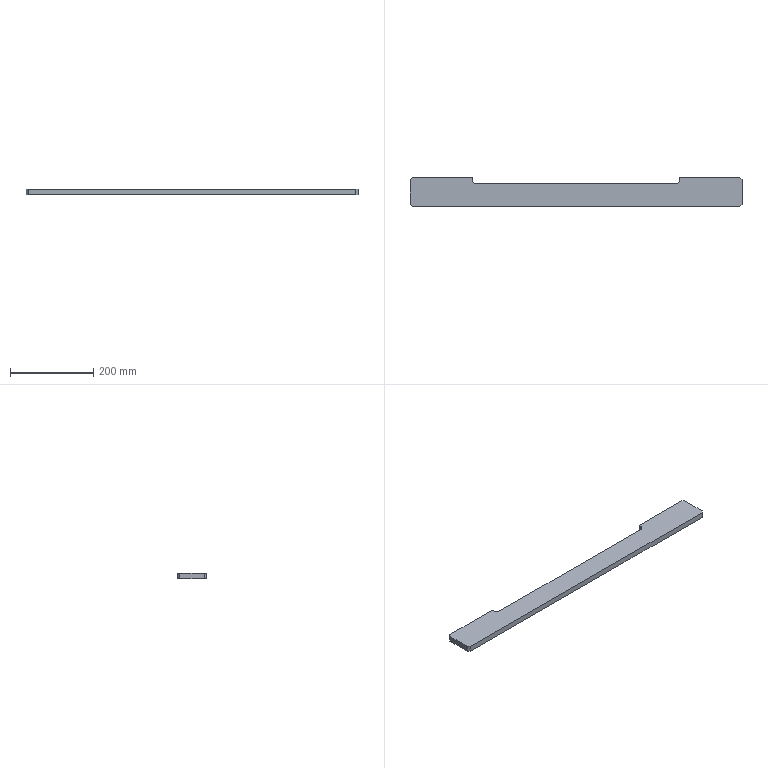Part | STEP file | 2012-06-08-01 | 1 solid | 16 faces | box 800 x 70 x 14 mm | volume 678901 mm3 | plane 14 | cylinder 2 | commonest cylinder face diameters 20 x2
STEP:
#1=CARTESIAN_POINT('',(0.,0.,0.));
#2=DIRECTION('',(0.,0.,1.));
#3=DIRECTION('',(1.,0.,0.));
#4=AXIS2_PLACEMENT_3D('',#1,#2,#3);
#5=CARTESIAN_POINT('',(-250.,35.,14.));
#6=VERTEX_POINT('',#5);
#7=CARTESIAN_POINT('',(-395.,35.,14.));
#8=VERTEX_POINT('',#7);
#9=CARTESIAN_POINT('',(-400.,35.,14.));
#10=DIRECTION('',(-1.,0.,0.));
#11=VECTOR('',#10,1.);
#12=LINE('',#9,#11);
#13=CARTESIAN_POINT('',(-400.,35.,14.));
#14=DIRECTION('',(0.,-1.,0.));
#15=DIRECTION('',(0.,0.,-1.));
#16=AXIS2_PLACEMENT_3D('',#13,#14,#15);
#17=PLANE('',#16);
#18=CARTESIAN_POINT('',(0.,0.));
#19=DIRECTION('',(0.,-1.));
#20=VECTOR('',#19,1.);
#21=LINE('',#18,#20);
#22=(GEOMETRIC_REPRESENTATION_CONTEXT(2)PARAMETRIC_REPRESENTATION_CONTEXT()REPRESENTATION_CONTEXT('',''));
#23=DEFINITIONAL_REPRESENTATION('',(#21),#22);
#24=PCURVE('',#17,#23);
#25=CARTESIAN_POINT('',(400.,-35.,14.));
#26=DIRECTION('',(0.,0.,1.));
#27=DIRECTION('',(1.,0.,0.));
#28=AXIS2_PLACEMENT_3D('',#25,#26,#27);
#29=PLANE('',#28);
#30=CARTESIAN_POINT('',(-800.,70.));
#31=DIRECTION('',(-1.,0.));
#32=VECTOR('',#31,1.);
#33=LINE('',#30,#32);
#34=(GEOMETRIC_REPRESENTATION_CONTEXT(2)PARAMETRIC_REPRESENTATION_CONTEXT()REPRESENTATION_CONTEXT('',''));
#35=DEFINITIONAL_REPRESENTATION('',(#33),#34);
#36=PCURVE('',#29,#35);
#37=SURFACE_CURVE('',#12,(#24,#36),.PCURVE_S1.);
#38=EDGE_CURVE('',#6,#8,#37,.T.);
#39=ORIENTED_EDGE('',*,*,#38,.F.);
#40=CARTESIAN_POINT('',(-250.,35.,0.));
#41=VERTEX_POINT('',#40);
#42=CARTESIAN_POINT('',(-250.,35.,-1.));
#43=DIRECTION('',(0.,0.,1.));
#44=VECTOR('',#43,1.);
#45=LINE('',#42,#44);
#46=CARTESIAN_POINT('',(15.,150.));
#47=DIRECTION('',(-1.,0.));
#48=VECTOR('',#47,1.);
#49=LINE('',#46,#48);
#50=(GEOMETRIC_REPRESENTATION_CONTEXT(2)PARAMETRIC_REPRESENTATION_CONTEXT()REPRESENTATION_CONTEXT('',''));
#51=DEFINITIONAL_REPRESENTATION('',(#49),#50);
#52=PCURVE('',#17,#51);
#53=CARTESIAN_POINT('',(-250.,35.,-1.));
#54=DIRECTION('',(-1.,0.,0.));
#55=DIRECTION('',(0.,0.,1.));
#56=AXIS2_PLACEMENT_3D('',#53,#54,#55);
#57=PLANE('',#56);
#58=CARTESIAN_POINT('',(0.,0.));
#59=DIRECTION('',(1.,0.));
#60=VECTOR('',#59,1.);
#61=LINE('',#58,#60);
#62=(GEOMETRIC_REPRESENTATION_CONTEXT(2)PARAMETRIC_REPRESENTATION_CONTEXT()REPRESENTATION_CONTEXT('',''));
#63=DEFINITIONAL_REPRESENTATION('',(#61),#62);
#64=PCURVE('',#57,#63);
#65=SURFACE_CURVE('',#45,(#52,#64),.PCURVE_S1.);
#66=EDGE_CURVE('',#41,#6,#65,.T.);
#67=ORIENTED_EDGE('',*,*,#66,.F.);
#68=CARTESIAN_POINT('',(-395.,35.,0.));
#69=VERTEX_POINT('',#68);
#70=CARTESIAN_POINT('',(-400.,35.,0.));
#71=DIRECTION('',(-1.,0.,0.));
#72=VECTOR('',#71,1.);
#73=LINE('',#70,#72);
#74=CARTESIAN_POINT('',(14.,0.));
#75=DIRECTION('',(0.,-1.));
#76=VECTOR('',#75,1.);
#77=LINE('',#74,#76);
#78=(GEOMETRIC_REPRESENTATION_CONTEXT(2)PARAMETRIC_REPRESENTATION_CONTEXT()REPRESENTATION_CONTEXT('',''));
#79=DEFINITIONAL_REPRESENTATION('',(#77),#78);
#80=PCURVE('',#17,#79);
#81=CARTESIAN_POINT('',(400.,-35.,0.));
#82=DIRECTION('',(0.,0.,1.));
#83=DIRECTION('',(1.,0.,0.));
#84=AXIS2_PLACEMENT_3D('',#81,#82,#83);
#85=PLANE('',#84);
#86=CARTESIAN_POINT('',(-800.,70.));
#87=DIRECTION('',(-1.,0.));
#88=VECTOR('',#87,1.);
#89=LINE('',#86,#88);
#90=(GEOMETRIC_REPRESENTATION_CONTEXT(2)PARAMETRIC_REPRESENTATION_CONTEXT()REPRESENTATION_CONTEXT('',''));
#91=DEFINITIONAL_REPRESENTATION('',(#89),#90);
#92=PCURVE('',#85,#91);
#93=SURFACE_CURVE('',#73,(#80,#92),.PCURVE_S1.);
#94=EDGE_CURVE('',#41,#69,#93,.T.);
#95=ORIENTED_EDGE('',*,*,#94,.T.);
#96=CARTESIAN_POINT('',(-395.,35.,14.));
#97=DIRECTION('',(0.,0.,1.));
#98=VECTOR('',#97,1.);
#99=LINE('',#96,#98);
#100=CARTESIAN_POINT('',(0.,5.));
#101=DIRECTION('',(-1.,0.));
#102=VECTOR('',#101,1.);
#103=LINE('',#100,#102);
#104=(GEOMETRIC_REPRESENTATION_CONTEXT(2)PARAMETRIC_REPRESENTATION_CONTEXT()REPRESENTATION_CONTEXT('',''));
#105=DEFINITIONAL_REPRESENTATION('',(#103),#104);
#106=PCURVE('',#17,#105);
#107=CARTESIAN_POINT('',(-400.,30.,14.));
#108=DIRECTION('',(0.7071,-0.7071,0.));
#109=DIRECTION('',(0.7071,0.7071,0.));
#110=AXIS2_PLACEMENT_3D('',#107,#108,#109);
#111=PLANE('',#110);
#112=CARTESIAN_POINT('',(7.071,0.));
#113=DIRECTION('',(0.,1.));
#114=VECTOR('',#113,1.);
#115=LINE('',#112,#114);
#116=(GEOMETRIC_REPRESENTATION_CONTEXT(2)PARAMETRIC_REPRESENTATION_CONTEXT()REPRESENTATION_CONTEXT('',''));
#117=DEFINITIONAL_REPRESENTATION('',(#115),#116);
#118=PCURVE('',#111,#117);
#119=SURFACE_CURVE('',#99,(#106,#118),.PCURVE_S1.);
#120=EDGE_CURVE('',#69,#8,#119,.T.);
#121=ORIENTED_EDGE('',*,*,#120,.T.);
#122=EDGE_LOOP('',(#39,#67,#95,#121));
#123=FACE_BOUND('',#122,.T.);
#124=ADVANCED_FACE('',(#123),#17,.F.);
#125=CARTESIAN_POINT('',(400.,-30.,14.));
#126=VERTEX_POINT('',#125);
#127=CARTESIAN_POINT('',(400.,30.,14.));
#128=VERTEX_POINT('',#127);
#129=CARTESIAN_POINT('',(400.,35.,14.));
#130=DIRECTION('',(0.,1.,0.));
#131=VECTOR('',#130,1.);
#132=LINE('',#129,#131);
#133=CARTESIAN_POINT('',(400.,35.,14.));
#134=DIRECTION('',(-1.,0.,0.));
#135=DIRECTION('',(0.,0.,1.));
#136=AXIS2_PLACEMENT_3D('',#133,#134,#135);
#137=PLANE('',#136);
#138=CARTESIAN_POINT('',(0.,0.));
#139=DIRECTION('',(0.,1.));
#140=VECTOR('',#139,1.);
#141=LINE('',#138,#140);
#142=(GEOMETRIC_REPRESENTATION_CONTEXT(2)PARAMETRIC_REPRESENTATION_CONTEXT()REPRESENTATION_CONTEXT('',''));
#143=DEFINITIONAL_REPRESENTATION('',(#141),#142);
#144=PCURVE('',#137,#143);
#145=CARTESIAN_POINT('',(0.,70.));
#146=DIRECTION('',(0.,1.));
#147=VECTOR('',#146,1.);
#148=LINE('',#145,#147);
#149=(GEOMETRIC_REPRESENTATION_CONTEXT(2)PARAMETRIC_REPRESENTATION_CONTEXT()REPRESENTATION_CONTEXT('',''));
#150=DEFINITIONAL_REPRESENTATION('',(#148),#149);
#151=PCURVE('',#29,#150);
#152=SURFACE_CURVE('',#132,(#144,#151),.PCURVE_S1.);
#153=EDGE_CURVE('',#126,#128,#152,.T.);
#154=ORIENTED_EDGE('',*,*,#153,.F.);
#155=CARTESIAN_POINT('',(400.,-30.,0.));
#156=VERTEX_POINT('',#155);
#157=CARTESIAN_POINT('',(400.,-30.,14.));
#158=DIRECTION('',(0.,0.,-1.));
#159=VECTOR('',#158,1.);
#160=LINE('',#157,#159);
#161=CARTESIAN_POINT('',(0.,-65.));
#162=DIRECTION('',(-1.,0.));
#163=VECTOR('',#162,1.);
#164=LINE('',#161,#163);
#165=(GEOMETRIC_REPRESENTATION_CONTEXT(2)PARAMETRIC_REPRESENTATION_CONTEXT()REPRESENTATION_CONTEXT('',''));
#166=DEFINITIONAL_REPRESENTATION('',(#164),#165);
#167=PCURVE('',#137,#166);
#168=CARTESIAN_POINT('',(400.,-30.,14.));
#169=DIRECTION('',(-0.7071,0.7071,0.));
#170=DIRECTION('',(-0.7071,-0.7071,0.));
#171=AXIS2_PLACEMENT_3D('',#168,#169,#170);
#172=PLANE('',#171);
#173=CARTESIAN_POINT('',(0.,0.));
#174=DIRECTION('',(0.,-1.));
#175=VECTOR('',#174,1.);
#176=LINE('',#173,#175);
#177=(GEOMETRIC_REPRESENTATION_CONTEXT(2)PARAMETRIC_REPRESENTATION_CONTEXT()REPRESENTATION_CONTEXT('',''));
#178=DEFINITIONAL_REPRESENTATION('',(#176),#177);
#179=PCURVE('',#172,#178);
#180=SURFACE_CURVE('',#160,(#167,#179),.PCURVE_S1.);
#181=EDGE_CURVE('',#126,#156,#180,.T.);
#182=ORIENTED_EDGE('',*,*,#181,.T.);
#183=CARTESIAN_POINT('',(400.,30.,0.));
#184=VERTEX_POINT('',#183);
#185=CARTESIAN_POINT('',(400.,35.,0.));
#186=DIRECTION('',(0.,1.,0.));
#187=VECTOR('',#186,1.);
#188=LINE('',#185,#187);
#189=CARTESIAN_POINT('',(-14.,0.));
#190=DIRECTION('',(0.,1.));
#191=VECTOR('',#190,1.);
#192=LINE('',#189,#191);
#193=(GEOMETRIC_REPRESENTATION_CONTEXT(2)PARAMETRIC_REPRESENTATION_CONTEXT()REPRESENTATION_CONTEXT('',''));
#194=DEFINITIONAL_REPRESENTATION('',(#192),#193);
#195=PCURVE('',#137,#194);
#196=CARTESIAN_POINT('',(0.,70.));
#197=DIRECTION('',(0.,1.));
#198=VECTOR('',#197,1.);
#199=LINE('',#196,#198);
#200=(GEOMETRIC_REPRESENTATION_CONTEXT(2)PARAMETRIC_REPRESENTATION_CONTEXT()REPRESENTATION_CONTEXT('',''));
#201=DEFINITIONAL_REPRESENTATION('',(#199),#200);
#202=PCURVE('',#85,#201);
#203=SURFACE_CURVE('',#188,(#195,#202),.PCURVE_S1.);
#204=EDGE_CURVE('',#156,#184,#203,.T.);
#205=ORIENTED_EDGE('',*,*,#204,.T.);
#206=CARTESIAN_POINT('',(400.,30.,14.));
#207=DIRECTION('',(0.,0.,1.));
#208=VECTOR('',#207,1.);
#209=LINE('',#206,#208);
#210=CARTESIAN_POINT('',(0.,-5.));
#211=DIRECTION('',(1.,0.));
#212=VECTOR('',#211,1.);
#213=LINE('',#210,#212);
#214=(GEOMETRIC_REPRESENTATION_CONTEXT(2)PARAMETRIC_REPRESENTATION_CONTEXT()REPRESENTATION_CONTEXT('',''));
#215=DEFINITIONAL_REPRESENTATION('',(#213),#214);
#216=PCURVE('',#137,#215);
#217=CARTESIAN_POINT('',(395.,35.,14.));
#218=DIRECTION('',(-0.7071,-0.7071,0.));
#219=DIRECTION('',(0.7071,-0.7071,0.));
#220=AXIS2_PLACEMENT_3D('',#217,#218,#219);
#221=PLANE('',#220);
#222=CARTESIAN_POINT('',(7.071,0.));
#223=DIRECTION('',(0.,1.));
#224=VECTOR('',#223,1.);
#225=LINE('',#222,#224);
#226=(GEOMETRIC_REPRESENTATION_CONTEXT(2)PARAMETRIC_REPRESENTATION_CONTEXT()REPRESENTATION_CONTEXT('',''));
#227=DEFINITIONAL_REPRESENTATION('',(#225),#226);
#228=PCURVE('',#221,#227);
#229=SURFACE_CURVE('',#209,(#216,#228),.PCURVE_S1.);
#230=EDGE_CURVE('',#184,#128,#229,.T.);
#231=ORIENTED_EDGE('',*,*,#230,.T.);
#232=EDGE_LOOP('',(#154,#182,#205,#231));
#233=FACE_BOUND('',#232,.T.);
#234=ADVANCED_FACE('',(#233),#137,.F.);
#235=CARTESIAN_POINT('',(395.,35.,0.));
#236=VERTEX_POINT('',#235);
#237=CARTESIAN_POINT('',(250.,35.,0.));
#238=VERTEX_POINT('',#237);
#239=CARTESIAN_POINT('',(-400.,35.,0.));
#240=DIRECTION('',(-1.,0.,0.));
#241=VECTOR('',#240,1.);
#242=LINE('',#239,#241);
#243=CARTESIAN_POINT('',(-400.,35.,14.));
#244=DIRECTION('',(0.,-1.,0.));
#245=DIRECTION('',(0.,0.,-1.));
#246=AXIS2_PLACEMENT_3D('',#243,#244,#245);
#247=PLANE('',#246);
#248=CARTESIAN_POINT('',(14.,0.));
#249=DIRECTION('',(0.,-1.));
#250=VECTOR('',#249,1.);
#251=LINE('',#248,#250);
#252=(GEOMETRIC_REPRESENTATION_CONTEXT(2)PARAMETRIC_REPRESENTATION_CONTEXT()REPRESENTATION_CONTEXT('',''));
#253=DEFINITIONAL_REPRESENTATION('',(#251),#252);
#254=PCURVE('',#247,#253);
#255=CARTESIAN_POINT('',(-800.,70.));
#256=DIRECTION('',(-1.,0.));
#257=VECTOR('',#256,1.);
#258=LINE('',#255,#257);
#259=(GEOMETRIC_REPRESENTATION_CONTEXT(2)PARAMETRIC_REPRESENTATION_CONTEXT()REPRESENTATION_CONTEXT('',''));
#260=DEFINITIONAL_REPRESENTATION('',(#258),#259);
#261=PCURVE('',#85,#260);
#262=SURFACE_CURVE('',#242,(#254,#261),.PCURVE_S1.);
#263=EDGE_CURVE('',#236,#238,#262,.T.);
#264=ORIENTED_EDGE('',*,*,#263,.T.);
#265=CARTESIAN_POINT('',(250.,35.,14.));
#266=VERTEX_POINT('',#265);
#267=CARTESIAN_POINT('',(250.,35.,-1.));
#268=DIRECTION('',(0.,0.,1.));
#269=VECTOR('',#268,1.);
#270=LINE('',#267,#269);
#271=CARTESIAN_POINT('',(15.,650.));
#272=DIRECTION('',(-1.,0.));
#273=VECTOR('',#272,1.);
#274=LINE('',#271,#273);
#275=(GEOMETRIC_REPRESENTATION_CONTEXT(2)PARAMETRIC_REPRESENTATION_CONTEXT()REPRESENTATION_CONTEXT('',''));
#276=DEFINITIONAL_REPRESENTATION('',(#274),#275);
#277=PCURVE('',#247,#276);
#278=CARTESIAN_POINT('',(250.,35.,-1.));
#279=DIRECTION('',(1.,0.,0.));
#280=DIRECTION('',(0.,0.,-1.));
#281=AXIS2_PLACEMENT_3D('',#278,#279,#280);
#282=PLANE('',#281);
#283=CARTESIAN_POINT('',(0.,0.));
#284=DIRECTION('',(-1.,0.));
#285=VECTOR('',#284,1.);
#286=LINE('',#283,#285);
#287=(GEOMETRIC_REPRESENTATION_CONTEXT(2)PARAMETRIC_REPRESENTATION_CONTEXT()REPRESENTATION_CONTEXT('',''));
#288=DEFINITIONAL_REPRESENTATION('',(#286),#287);
#289=PCURVE('',#282,#288);
#290=SURFACE_CURVE('',#270,(#277,#289),.PCURVE_S1.);
#291=EDGE_CURVE('',#238,#266,#290,.T.);
#292=ORIENTED_EDGE('',*,*,#291,.T.);
#293=CARTESIAN_POINT('',(395.,35.,14.));
#294=VERTEX_POINT('',#293);
#295=CARTESIAN_POINT('',(-400.,35.,14.));
#296=DIRECTION('',(-1.,0.,0.));
#297=VECTOR('',#296,1.);
#298=LINE('',#295,#297);
#299=CARTESIAN_POINT('',(0.,0.));
#300=DIRECTION('',(0.,-1.));
#301=VECTOR('',#300,1.);
#302=LINE('',#299,#301);
#303=(GEOMETRIC_REPRESENTATION_CONTEXT(2)PARAMETRIC_REPRESENTATION_CONTEXT()REPRESENTATION_CONTEXT('',''));
#304=DEFINITIONAL_REPRESENTATION('',(#302),#303);
#305=PCURVE('',#247,#304);
#306=CARTESIAN_POINT('',(-800.,70.));
#307=DIRECTION('',(-1.,0.));
#308=VECTOR('',#307,1.);
#309=LINE('',#306,#308);
#310=(GEOMETRIC_REPRESENTATION_CONTEXT(2)PARAMETRIC_REPRESENTATION_CONTEXT()REPRESENTATION_CONTEXT('',''));
#311=DEFINITIONAL_REPRESENTATION('',(#309),#310);
#312=PCURVE('',#29,#311);
#313=SURFACE_CURVE('',#298,(#305,#312),.PCURVE_S1.);
#314=EDGE_CURVE('',#294,#266,#313,.T.);
#315=ORIENTED_EDGE('',*,*,#314,.F.);
#316=CARTESIAN_POINT('',(395.,35.,14.));
#317=DIRECTION('',(0.,0.,-1.));
#318=VECTOR('',#317,1.);
#319=LINE('',#316,#318);
#320=CARTESIAN_POINT('',(0.,795.));
#321=DIRECTION('',(1.,0.));
#322=VECTOR('',#321,1.);
#323=LINE('',#320,#322);
#324=(GEOMETRIC_REPRESENTATION_CONTEXT(2)PARAMETRIC_REPRESENTATION_CONTEXT()REPRESENTATION_CONTEXT('',''));
#325=DEFINITIONAL_REPRESENTATION('',(#323),#324);
#326=PCURVE('',#247,#325);
#327=CARTESIAN_POINT('',(0.,0.));
#328=DIRECTION('',(0.,-1.));
#329=VECTOR('',#328,1.);
#330=LINE('',#327,#329);
#331=(GEOMETRIC_REPRESENTATION_CONTEXT(2)PARAMETRIC_REPRESENTATION_CONTEXT()REPRESENTATION_CONTEXT('',''));
#332=DEFINITIONAL_REPRESENTATION('',(#330),#331);
#333=PCURVE('',#221,#332);
#334=SURFACE_CURVE('',#319,(#326,#333),.PCURVE_S1.);
#335=EDGE_CURVE('',#294,#236,#334,.T.);
#336=ORIENTED_EDGE('',*,*,#335,.T.);
#337=EDGE_LOOP('',(#264,#292,#315,#336));
#338=FACE_BOUND('',#337,.T.);
#339=ADVANCED_FACE('',(#338),#247,.F.);
#340=CARTESIAN_POINT('',(-400.,30.,0.));
#341=VERTEX_POINT('',#340);
#342=CARTESIAN_POINT('',(-400.,-30.,0.));
#343=VERTEX_POINT('',#342);
#344=CARTESIAN_POINT('',(-400.,35.,0.));
#345=DIRECTION('',(0.,-1.,0.));
#346=VECTOR('',#345,1.);
#347=LINE('',#344,#346);
#348=CARTESIAN_POINT('',(-400.,35.,14.));
#349=DIRECTION('',(1.,0.,0.));
#350=DIRECTION('',(0.,0.,-1.));
#351=AXIS2_PLACEMENT_3D('',#348,#349,#350);
#352=PLANE('',#351);
#353=CARTESIAN_POINT('',(14.,0.));
#354=DIRECTION('',(0.,-1.));
#355=VECTOR('',#354,1.);
#356=LINE('',#353,#355);
#357=(GEOMETRIC_REPRESENTATION_CONTEXT(2)PARAMETRIC_REPRESENTATION_CONTEXT()REPRESENTATION_CONTEXT('',''));
#358=DEFINITIONAL_REPRESENTATION('',(#356),#357);
#359=PCURVE('',#352,#358);
#360=CARTESIAN_POINT('',(-800.,70.));
#361=DIRECTION('',(0.,-1.));
#362=VECTOR('',#361,1.);
#363=LINE('',#360,#362);
#364=(GEOMETRIC_REPRESENTATION_CONTEXT(2)PARAMETRIC_REPRESENTATION_CONTEXT()REPRESENTATION_CONTEXT('',''));
#365=DEFINITIONAL_REPRESENTATION('',(#363),#364);
#366=PCURVE('',#85,#365);
#367=SURFACE_CURVE('',#347,(#359,#366),.PCURVE_S1.);
#368=EDGE_CURVE('',#341,#343,#367,.T.);
#369=ORIENTED_EDGE('',*,*,#368,.T.);
#370=CARTESIAN_POINT('',(-400.,-30.,14.));
#371=VERTEX_POINT('',#370);
#372=CARTESIAN_POINT('',(-400.,-30.,14.));
#373=DIRECTION('',(0.,0.,1.));
#374=VECTOR('',#373,1.);
#375=LINE('',#372,#374);
#376=CARTESIAN_POINT('',(0.,-65.));
#377=DIRECTION('',(-1.,0.));
#378=VECTOR('',#377,1.);
#379=LINE('',#376,#378);
#380=(GEOMETRIC_REPRESENTATION_CONTEXT(2)PARAMETRIC_REPRESENTATION_CONTEXT()REPRESENTATION_CONTEXT('',''));
#381=DEFINITIONAL_REPRESENTATION('',(#379),#380);
#382=PCURVE('',#352,#381);
#383=CARTESIAN_POINT('',(-395.,-35.,14.));
#384=DIRECTION('',(0.7071,0.7071,0.));
#385=DIRECTION('',(-0.7071,0.7071,0.));
#386=AXIS2_PLACEMENT_3D('',#383,#384,#385);
#387=PLANE('',#386);
#388=CARTESIAN_POINT('',(7.071,0.));
#389=DIRECTION('',(0.,1.));
#390=VECTOR('',#389,1.);
#391=LINE('',#388,#390);
#392=(GEOMETRIC_REPRESENTATION_CONTEXT(2)PARAMETRIC_REPRESENTATION_CONTEXT()REPRESENTATION_CONTEXT('',''));
#393=DEFINITIONAL_REPRESENTATION('',(#391),#392);
#394=PCURVE('',#387,#393);
#395=SURFACE_CURVE('',#375,(#382,#394),.PCURVE_S1.);
#396=EDGE_CURVE('',#343,#371,#395,.T.);
#397=ORIENTED_EDGE('',*,*,#396,.T.);
#398=CARTESIAN_POINT('',(-400.,30.,14.));
#399=VERTEX_POINT('',#398);
#400=CARTESIAN_POINT('',(-400.,35.,14.));
#401=DIRECTION('',(0.,-1.,0.));
#402=VECTOR('',#401,1.);
#403=LINE('',#400,#402);
#404=CARTESIAN_POINT('',(0.,0.));
#405=DIRECTION('',(0.,-1.));
#406=VECTOR('',#405,1.);
#407=LINE('',#404,#406);
#408=(GEOMETRIC_REPRESENTATION_CONTEXT(2)PARAMETRIC_REPRESENTATION_CONTEXT()REPRESENTATION_CONTEXT('',''));
#409=DEFINITIONAL_REPRESENTATION('',(#407),#408);
#410=PCURVE('',#352,#409);
#411=CARTESIAN_POINT('',(-800.,70.));
#412=DIRECTION('',(0.,-1.));
#413=VECTOR('',#412,1.);
#414=LINE('',#411,#413);
#415=(GEOMETRIC_REPRESENTATION_CONTEXT(2)PARAMETRIC_REPRESENTATION_CONTEXT()REPRESENTATION_CONTEXT('',''));
#416=DEFINITIONAL_REPRESENTATION('',(#414),#415);
#417=PCURVE('',#29,#416);
#418=SURFACE_CURVE('',#403,(#410,#417),.PCURVE_S1.);
#419=EDGE_CURVE('',#399,#371,#418,.T.);
#420=ORIENTED_EDGE('',*,*,#419,.F.);
#421=CARTESIAN_POINT('',(-400.,30.,14.));
#422=DIRECTION('',(0.,0.,-1.));
#423=VECTOR('',#422,1.);
#424=LINE('',#421,#423);
#425=CARTESIAN_POINT('',(0.,-5.));
#426=DIRECTION('',(1.,0.));
#427=VECTOR('',#426,1.);
#428=LINE('',#425,#427);
#429=(GEOMETRIC_REPRESENTATION_CONTEXT(2)PARAMETRIC_REPRESENTATION_CONTEXT()REPRESENTATION_CONTEXT('',''));
#430=DEFINITIONAL_REPRESENTATION('',(#428),#429);
#431=PCURVE('',#352,#430);
#432=CARTESIAN_POINT('',(0.,0.));
#433=DIRECTION('',(0.,-1.));
#434=VECTOR('',#433,1.);
#435=LINE('',#432,#434);
#436=(GEOMETRIC_REPRESENTATION_CONTEXT(2)PARAMETRIC_REPRESENTATION_CONTEXT()REPRESENTATION_CONTEXT('',''));
#437=DEFINITIONAL_REPRESENTATION('',(#435),#436);
#438=PCURVE('',#111,#437);
#439=SURFACE_CURVE('',#424,(#431,#438),.PCURVE_S1.);
#440=EDGE_CURVE('',#399,#341,#439,.T.);
#441=ORIENTED_EDGE('',*,*,#440,.T.);
#442=EDGE_LOOP('',(#369,#397,#420,#441));
#443=FACE_BOUND('',#442,.T.);
#444=ADVANCED_FACE('',(#443),#352,.F.);
#445=CARTESIAN_POINT('',(-395.,-35.,14.));
#446=VERTEX_POINT('',#445);
#447=CARTESIAN_POINT('',(395.,-35.,14.));
#448=VERTEX_POINT('',#447);
#449=CARTESIAN_POINT('',(-400.,-35.,14.));
#450=DIRECTION('',(1.,0.,0.));
#451=VECTOR('',#450,1.);
#452=LINE('',#449,#451);
#453=CARTESIAN_POINT('',(-400.,-35.,14.));
#454=DIRECTION('',(0.,1.,0.));
#455=DIRECTION('',(0.,0.,1.));
#456=AXIS2_PLACEMENT_3D('',#453,#454,#455);
#457=PLANE('',#456);
#458=CARTESIAN_POINT('',(0.,0.));
#459=DIRECTION('',(0.,1.));
#460=VECTOR('',#459,1.);
#461=LINE('',#458,#460);
#462=(GEOMETRIC_REPRESENTATION_CONTEXT(2)PARAMETRIC_REPRESENTATION_CONTEXT()REPRESENTATION_CONTEXT('',''));
#463=DEFINITIONAL_REPRESENTATION('',(#461),#462);
#464=PCURVE('',#457,#463);
#465=CARTESIAN_POINT('',(-800.,0.));
#466=DIRECTION('',(1.,0.));
#467=VECTOR('',#466,1.);
#468=LINE('',#465,#467);
#469=(GEOMETRIC_REPRESENTATION_CONTEXT(2)PARAMETRIC_REPRESENTATION_CONTEXT()REPRESENTATION_CONTEXT('',''));
#470=DEFINITIONAL_REPRESENTATION('',(#468),#469);
#471=PCURVE('',#29,#470);
#472=SURFACE_CURVE('',#452,(#464,#471),.PCURVE_S1.);
#473=EDGE_CURVE('',#446,#448,#472,.T.);
#474=ORIENTED_EDGE('',*,*,#473,.F.);
#475=CARTESIAN_POINT('',(-395.,-35.,0.));
#476=VERTEX_POINT('',#475);
#477=CARTESIAN_POINT('',(-395.,-35.,14.));
#478=DIRECTION('',(0.,0.,-1.));
#479=VECTOR('',#478,1.);
#480=LINE('',#477,#479);
#481=CARTESIAN_POINT('',(0.,5.));
#482=DIRECTION('',(-1.,0.));
#483=VECTOR('',#482,1.);
#484=LINE('',#481,#483);
#485=(GEOMETRIC_REPRESENTATION_CONTEXT(2)PARAMETRIC_REPRESENTATION_CONTEXT()REPRESENTATION_CONTEXT('',''));
#486=DEFINITIONAL_REPRESENTATION('',(#484),#485);
#487=PCURVE('',#457,#486);
#488=CARTESIAN_POINT('',(0.,0.));
#489=DIRECTION('',(0.,-1.));
#490=VECTOR('',#489,1.);
#491=LINE('',#488,#490);
#492=(GEOMETRIC_REPRESENTATION_CONTEXT(2)PARAMETRIC_REPRESENTATION_CONTEXT()REPRESENTATION_CONTEXT('',''));
#493=DEFINITIONAL_REPRESENTATION('',(#491),#492);
#494=PCURVE('',#387,#493);
#495=SURFACE_CURVE('',#480,(#487,#494),.PCURVE_S1.);
#496=EDGE_CURVE('',#446,#476,#495,.T.);
#497=ORIENTED_EDGE('',*,*,#496,.T.);
#498=CARTESIAN_POINT('',(395.,-35.,0.));
#499=VERTEX_POINT('',#498);
#500=CARTESIAN_POINT('',(-400.,-35.,0.));
#501=DIRECTION('',(1.,0.,0.));
#502=VECTOR('',#501,1.);
#503=LINE('',#500,#502);
#504=CARTESIAN_POINT('',(-14.,0.));
#505=DIRECTION('',(0.,1.));
#506=VECTOR('',#505,1.);
#507=LINE('',#504,#506);
#508=(GEOMETRIC_REPRESENTATION_CONTEXT(2)PARAMETRIC_REPRESENTATION_CONTEXT()REPRESENTATION_CONTEXT('',''));
#509=DEFINITIONAL_REPRESENTATION('',(#507),#508);
#510=PCURVE('',#457,#509);
#511=CARTESIAN_POINT('',(-800.,0.));
#512=DIRECTION('',(1.,0.));
#513=VECTOR('',#512,1.);
#514=LINE('',#511,#513);
#515=(GEOMETRIC_REPRESENTATION_CONTEXT(2)PARAMETRIC_REPRESENTATION_CONTEXT()REPRESENTATION_CONTEXT('',''));
#516=DEFINITIONAL_REPRESENTATION('',(#514),#515);
#517=PCURVE('',#85,#516);
#518=SURFACE_CURVE('',#503,(#510,#517),.PCURVE_S1.);
#519=EDGE_CURVE('',#476,#499,#518,.T.);
#520=ORIENTED_EDGE('',*,*,#519,.T.);
#521=CARTESIAN_POINT('',(395.,-35.,14.));
#522=DIRECTION('',(0.,0.,1.));
#523=VECTOR('',#522,1.);
#524=LINE('',#521,#523);
#525=CARTESIAN_POINT('',(0.,795.));
#526=DIRECTION('',(1.,0.));
#527=VECTOR('',#526,1.);
#528=LINE('',#525,#527);
#529=(GEOMETRIC_REPRESENTATION_CONTEXT(2)PARAMETRIC_REPRESENTATION_CONTEXT()REPRESENTATION_CONTEXT('',''));
#530=DEFINITIONAL_REPRESENTATION('',(#528),#529);
#531=PCURVE('',#457,#530);
#532=CARTESIAN_POINT('',(7.071,0.));
#533=DIRECTION('',(0.,1.));
#534=VECTOR('',#533,1.);
#535=LINE('',#532,#534);
#536=(GEOMETRIC_REPRESENTATION_CONTEXT(2)PARAMETRIC_REPRESENTATION_CONTEXT()REPRESENTATION_CONTEXT('',''));
#537=DEFINITIONAL_REPRESENTATION('',(#535),#536);
#538=PCURVE('',#172,#537);
#539=SURFACE_CURVE('',#524,(#531,#538),.PCURVE_S1.);
#540=EDGE_CURVE('',#499,#448,#539,.T.);
#541=ORIENTED_EDGE('',*,*,#540,.T.);
#542=EDGE_LOOP('',(#474,#497,#520,#541));
#543=FACE_BOUND('',#542,.T.);
#544=ADVANCED_FACE('',(#543),#457,.F.);
#545=CARTESIAN_POINT('',(-250.,30.,14.));
#546=VERTEX_POINT('',#545);
#547=CARTESIAN_POINT('',(-250.,35.,14.));
#548=DIRECTION('',(0.,-1.,0.));
#549=VECTOR('',#548,1.);
#550=LINE('',#547,#549);
#551=CARTESIAN_POINT('',(-650.,70.));
#552=DIRECTION('',(0.,-1.));
#553=VECTOR('',#552,1.);
#554=LINE('',#551,#553);
#555=(GEOMETRIC_REPRESENTATION_CONTEXT(2)PARAMETRIC_REPRESENTATION_CONTEXT()REPRESENTATION_CONTEXT('',''));
#556=DEFINITIONAL_REPRESENTATION('',(#554),#555);
#557=PCURVE('',#29,#556);
#558=CARTESIAN_POINT('',(15.,0.));
#559=DIRECTION('',(0.,-1.));
#560=VECTOR('',#559,1.);
#561=LINE('',#558,#560);
#562=(GEOMETRIC_REPRESENTATION_CONTEXT(2)PARAMETRIC_REPRESENTATION_CONTEXT()REPRESENTATION_CONTEXT('',''));
#563=DEFINITIONAL_REPRESENTATION('',(#561),#562);
#564=PCURVE('',#57,#563);
#565=SURFACE_CURVE('',#550,(#557,#564),.PCURVE_S1.);
#566=EDGE_CURVE('',#6,#546,#565,.T.);
#567=ORIENTED_EDGE('',*,*,#566,.F.);
#568=ORIENTED_EDGE('',*,*,#38,.T.);
#569=CARTESIAN_POINT('',(-32.5,397.5,14.));
#570=DIRECTION('',(-0.7071,-0.7071,0.));
#571=VECTOR('',#570,1.);
#572=LINE('',#569,#571);
#573=CARTESIAN_POINT('',(-432.5,432.5));
#574=DIRECTION('',(-0.7071,-0.7071));
#575=VECTOR('',#574,1.);
#576=LINE('',#573,#575);
#577=(GEOMETRIC_REPRESENTATION_CONTEXT(2)PARAMETRIC_REPRESENTATION_CONTEXT()REPRESENTATION_CONTEXT('',''));
#578=DEFINITIONAL_REPRESENTATION('',(#576),#577);
#579=PCURVE('',#29,#578);
#580=CARTESIAN_POINT('',(519.723,0.));
#581=DIRECTION('',(-1.,0.));
#582=VECTOR('',#581,1.);
#583=LINE('',#580,#582);
#584=(GEOMETRIC_REPRESENTATION_CONTEXT(2)PARAMETRIC_REPRESENTATION_CONTEXT()REPRESENTATION_CONTEXT('',''));
#585=DEFINITIONAL_REPRESENTATION('',(#583),#584);
#586=PCURVE('',#111,#585);
#587=SURFACE_CURVE('',#572,(#579,#586),.PCURVE_S1.);
#588=EDGE_CURVE('',#8,#399,#587,.T.);
#589=ORIENTED_EDGE('',*,*,#588,.T.);
#590=ORIENTED_EDGE('',*,*,#419,.T.);
#591=CARTESIAN_POINT('',(2.5,-432.5,14.));
#592=DIRECTION('',(0.7071,-0.7071,0.));
#593=VECTOR('',#592,1.);
#594=LINE('',#591,#593);
#595=CARTESIAN_POINT('',(-397.5,-397.5));
#596=DIRECTION('',(0.7071,-0.7071));
#597=VECTOR('',#596,1.);
#598=LINE('',#595,#597);
#599=(GEOMETRIC_REPRESENTATION_CONTEXT(2)PARAMETRIC_REPRESENTATION_CONTEXT()REPRESENTATION_CONTEXT('',''));
#600=DEFINITIONAL_REPRESENTATION('',(#598),#599);
#601=PCURVE('',#29,#600);
#602=CARTESIAN_POINT('',(-562.15,0.));
#603=DIRECTION('',(-1.,0.));
#604=VECTOR('',#603,1.);
#605=LINE('',#602,#604);
#606=(GEOMETRIC_REPRESENTATION_CONTEXT(2)PARAMETRIC_REPRESENTATION_CONTEXT()REPRESENTATION_CONTEXT('',''));
#607=DEFINITIONAL_REPRESENTATION('',(#605),#606);
#608=PCURVE('',#387,#607);
#609=SURFACE_CURVE('',#594,(#601,#608),.PCURVE_S1.);
#610=EDGE_CURVE('',#371,#446,#609,.T.);
#611=ORIENTED_EDGE('',*,*,#610,.T.);
#612=ORIENTED_EDGE('',*,*,#473,.T.);
#613=CARTESIAN_POINT('',(397.5,-32.5,14.));
#614=DIRECTION('',(0.7071,0.7071,0.));
#615=VECTOR('',#614,1.);
#616=LINE('',#613,#615);
#617=CARTESIAN_POINT('',(-2.5,2.5));
#618=DIRECTION('',(0.7071,0.7071));
#619=VECTOR('',#618,1.);
#620=LINE('',#617,#619);
#621=(GEOMETRIC_REPRESENTATION_CONTEXT(2)PARAMETRIC_REPRESENTATION_CONTEXT()REPRESENTATION_CONTEXT('',''));
#622=DEFINITIONAL_REPRESENTATION('',(#620),#621);
#623=PCURVE('',#29,#622);
#624=CARTESIAN_POINT('',(3.536,0.));
#625=DIRECTION('',(-1.,0.));
#626=VECTOR('',#625,1.);
#627=LINE('',#624,#626);
#628=(GEOMETRIC_REPRESENTATION_CONTEXT(2)PARAMETRIC_REPRESENTATION_CONTEXT()REPRESENTATION_CONTEXT('',''));
#629=DEFINITIONAL_REPRESENTATION('',(#627),#628);
#630=PCURVE('',#172,#629);
#631=SURFACE_CURVE('',#616,(#623,#630),.PCURVE_S1.);
#632=EDGE_CURVE('',#448,#126,#631,.T.);
#633=ORIENTED_EDGE('',*,*,#632,.T.);
#634=ORIENTED_EDGE('',*,*,#153,.T.);
#635=CARTESIAN_POINT('',(432.5,-2.5,14.));
#636=DIRECTION('',(-0.7071,0.7071,0.));
#637=VECTOR('',#636,1.);
#638=LINE('',#635,#637);
#639=CARTESIAN_POINT('',(32.5,32.5));
#640=DIRECTION('',(-0.7071,0.7071));
#641=VECTOR('',#640,1.);
#642=LINE('',#639,#641);
#643=(GEOMETRIC_REPRESENTATION_CONTEXT(2)PARAMETRIC_REPRESENTATION_CONTEXT()REPRESENTATION_CONTEXT('',''));
#644=DEFINITIONAL_REPRESENTATION('',(#642),#643);
#645=PCURVE('',#29,#644);
#646=CARTESIAN_POINT('',(53.033,0.));
#647=DIRECTION('',(-1.,0.));
#648=VECTOR('',#647,1.);
#649=LINE('',#646,#648);
#650=(GEOMETRIC_REPRESENTATION_CONTEXT(2)PARAMETRIC_REPRESENTATION_CONTEXT()REPRESENTATION_CONTEXT('',''));
#651=DEFINITIONAL_REPRESENTATION('',(#649),#650);
#652=PCURVE('',#221,#651);
#653=SURFACE_CURVE('',#638,(#645,#652),.PCURVE_S1.);
#654=EDGE_CURVE('',#128,#294,#653,.T.);
#655=ORIENTED_EDGE('',*,*,#654,.T.);
#656=ORIENTED_EDGE('',*,*,#314,.T.);
#657=CARTESIAN_POINT('',(250.,30.,14.));
#658=VERTEX_POINT('',#657);
#659=CARTESIAN_POINT('',(250.,35.,14.));
#660=DIRECTION('',(0.,1.,0.));
#661=VECTOR('',#660,1.);
#662=LINE('',#659,#661);
#663=CARTESIAN_POINT('',(-150.,70.));
#664=DIRECTION('',(0.,1.));
#665=VECTOR('',#664,1.);
#666=LINE('',#663,#665);
#667=(GEOMETRIC_REPRESENTATION_CONTEXT(2)PARAMETRIC_REPRESENTATION_CONTEXT()REPRESENTATION_CONTEXT('',''));
#668=DEFINITIONAL_REPRESENTATION('',(#666),#667);
#669=PCURVE('',#29,#668);
#670=CARTESIAN_POINT('',(-15.,0.));
#671=DIRECTION('',(0.,1.));
#672=VECTOR('',#671,1.);
#673=LINE('',#670,#672);
#674=(GEOMETRIC_REPRESENTATION_CONTEXT(2)PARAMETRIC_REPRESENTATION_CONTEXT()REPRESENTATION_CONTEXT('',''));
#675=DEFINITIONAL_REPRESENTATION('',(#673),#674);
#676=PCURVE('',#282,#675);
#677=SURFACE_CURVE('',#662,(#669,#676),.PCURVE_S1.);
#678=EDGE_CURVE('',#658,#266,#677,.T.);
#679=ORIENTED_EDGE('',*,*,#678,.F.);
#680=CARTESIAN_POINT('',(240.,20.,14.));
#681=VERTEX_POINT('',#680);
#682=CARTESIAN_POINT('',(240.,30.,14.));
#683=DIRECTION('',(0.,0.,-1.));
#684=DIRECTION('',(1.,0.,0.));
#685=AXIS2_PLACEMENT_3D('',#682,#683,#684);
#686=CIRCLE('',#685,10.);
#687=CARTESIAN_POINT('',(-150.,65.));
#688=CARTESIAN_POINT('',(-150.,47.679));
#689=CARTESIAN_POINT('',(-165.,56.34));
#690=CARTESIAN_POINT('',(-180.,65.));
#691=CARTESIAN_POINT('',(-165.,73.66));
#692=CARTESIAN_POINT('',(-150.,82.321));
#693=CARTESIAN_POINT('',(-150.,65.));
#694=(BOUNDED_CURVE()B_SPLINE_CURVE(2,(#687,#688,#689,#690,#691,#692,#693),.UNSPECIFIED.,.T.,.F.)B_SPLINE_CURVE_WITH_KNOTS((1,2,2,2,2,1),(-2.094,0.,2.094,4.189,6.283,8.378),.UNSPECIFIED.)CURVE()GEOMETRIC_REPRESENTATION_ITEM()RATIONAL_B_SPLINE_CURVE((1.,0.5,1.,0.5,1.,0.5,1.))REPRESENTATION_ITEM(''));
#695=(GEOMETRIC_REPRESENTATION_CONTEXT(2)PARAMETRIC_REPRESENTATION_CONTEXT()REPRESENTATION_CONTEXT('',''));
#696=DEFINITIONAL_REPRESENTATION('',(#694),#695);
#697=PCURVE('',#29,#696);
#698=CARTESIAN_POINT('',(240.,30.,-1.));
#699=DIRECTION('',(0.,0.,-1.));
#700=DIRECTION('',(-1.,0.,0.));
#701=AXIS2_PLACEMENT_3D('',#698,#699,#700);
#702=CYLINDRICAL_SURFACE('',#701,10.);
#703=CARTESIAN_POINT('',(3.142,-15.));
#704=DIRECTION('',(1.,0.));
#705=VECTOR('',#704,1.);
#706=LINE('',#703,#705);
#707=(GEOMETRIC_REPRESENTATION_CONTEXT(2)PARAMETRIC_REPRESENTATION_CONTEXT()REPRESENTATION_CONTEXT('',''));
#708=DEFINITIONAL_REPRESENTATION('',(#706),#707);
#709=PCURVE('',#702,#708);
#710=SURFACE_CURVE('',#686,(#697,#709),.PCURVE_S1.);
#711=EDGE_CURVE('',#658,#681,#710,.T.);
#712=ORIENTED_EDGE('',*,*,#711,.T.);
#713=CARTESIAN_POINT('',(-240.,20.,14.));
#714=VERTEX_POINT('',#713);
#715=CARTESIAN_POINT('',(-250.,20.,14.));
#716=DIRECTION('',(1.,0.,0.));
#717=VECTOR('',#716,1.);
#718=LINE('',#715,#717);
#719=CARTESIAN_POINT('',(-650.,55.));
#720=DIRECTION('',(1.,0.));
#721=VECTOR('',#720,1.);
#722=LINE('',#719,#721);
#723=(GEOMETRIC_REPRESENTATION_CONTEXT(2)PARAMETRIC_REPRESENTATION_CONTEXT()REPRESENTATION_CONTEXT('',''));
#724=DEFINITIONAL_REPRESENTATION('',(#722),#723);
#725=PCURVE('',#29,#724);
#726=CARTESIAN_POINT('',(-250.,20.,-1.));
#727=DIRECTION('',(0.,-1.,0.));
#728=DIRECTION('',(1.,0.,0.));
#729=AXIS2_PLACEMENT_3D('',#726,#727,#728);
#730=PLANE('',#729);
#731=CARTESIAN_POINT('',(0.,15.));
#732=DIRECTION('',(1.,0.));
#733=VECTOR('',#732,1.);
#734=LINE('',#731,#733);
#735=(GEOMETRIC_REPRESENTATION_CONTEXT(2)PARAMETRIC_REPRESENTATION_CONTEXT()REPRESENTATION_CONTEXT('',''));
#736=DEFINITIONAL_REPRESENTATION('',(#734),#735);
#737=PCURVE('',#730,#736);
#738=SURFACE_CURVE('',#718,(#725,#737),.PCURVE_S1.);
#739=EDGE_CURVE('',#714,#681,#738,.T.);
#740=ORIENTED_EDGE('',*,*,#739,.F.);
#741=CARTESIAN_POINT('',(-240.,30.,14.));
#742=DIRECTION('',(0.,0.,-1.));
#743=DIRECTION('',(1.,0.,0.));
#744=AXIS2_PLACEMENT_3D('',#741,#742,#743);
#745=CIRCLE('',#744,10.);
#746=CARTESIAN_POINT('',(-630.,65.));
#747=CARTESIAN_POINT('',(-630.,47.679));
#748=CARTESIAN_POINT('',(-645.,56.34));
#749=CARTESIAN_POINT('',(-660.,65.));
#750=CARTESIAN_POINT('',(-645.,73.66));
#751=CARTESIAN_POINT('',(-630.,82.321));
#752=CARTESIAN_POINT('',(-630.,65.));
#753=(BOUNDED_CURVE()B_SPLINE_CURVE(2,(#746,#747,#748,#749,#750,#751,#752),.UNSPECIFIED.,.T.,.F.)B_SPLINE_CURVE_WITH_KNOTS((1,2,2,2,2,1),(-2.094,0.,2.094,4.189,6.283,8.378),.UNSPECIFIED.)CURVE()GEOMETRIC_REPRESENTATION_ITEM()RATIONAL_B_SPLINE_CURVE((1.,0.5,1.,0.5,1.,0.5,1.))REPRESENTATION_ITEM(''));
#754=(GEOMETRIC_REPRESENTATION_CONTEXT(2)PARAMETRIC_REPRESENTATION_CONTEXT()REPRESENTATION_CONTEXT('',''));
#755=DEFINITIONAL_REPRESENTATION('',(#753),#754);
#756=PCURVE('',#29,#755);
#757=CARTESIAN_POINT('',(-240.,30.,-1.));
#758=DIRECTION('',(0.,0.,-1.));
#759=DIRECTION('',(-1.,0.,0.));
#760=AXIS2_PLACEMENT_3D('',#757,#758,#759);
#761=CYLINDRICAL_SURFACE('',#760,10.);
#762=CARTESIAN_POINT('',(3.142,-15.));
#763=DIRECTION('',(1.,0.));
#764=VECTOR('',#763,1.);
#765=LINE('',#762,#764);
#766=(GEOMETRIC_REPRESENTATION_CONTEXT(2)PARAMETRIC_REPRESENTATION_CONTEXT()REPRESENTATION_CONTEXT('',''));
#767=DEFINITIONAL_REPRESENTATION('',(#765),#766);
#768=PCURVE('',#761,#767);
#769=SURFACE_CURVE('',#745,(#756,#768),.PCURVE_S1.);
#770=EDGE_CURVE('',#714,#546,#769,.T.);
#771=ORIENTED_EDGE('',*,*,#770,.T.);
#772=EDGE_LOOP('',(#567,#568,#589,#590,#611,#612,#633,#634,#655,#656,#679,#712,#740,#771));
#773=FACE_BOUND('',#772,.T.);
#774=ADVANCED_FACE('',(#773),#29,.T.);
#775=ORIENTED_EDGE('',*,*,#94,.F.);
#776=CARTESIAN_POINT('',(-250.,30.,0.));
#777=VERTEX_POINT('',#776);
#778=CARTESIAN_POINT('',(-250.,-35.,0.));
#779=DIRECTION('',(0.,-1.,0.));
#780=VECTOR('',#779,1.);
#781=LINE('',#778,#780);
#782=CARTESIAN_POINT('',(-650.,0.));
#783=DIRECTION('',(0.,-1.));
#784=VECTOR('',#783,1.);
#785=LINE('',#782,#784);
#786=(GEOMETRIC_REPRESENTATION_CONTEXT(2)PARAMETRIC_REPRESENTATION_CONTEXT()REPRESENTATION_CONTEXT('',''));
#787=DEFINITIONAL_REPRESENTATION('',(#785),#786);
#788=PCURVE('',#85,#787);
#789=CARTESIAN_POINT('',(1.,-70.));
#790=DIRECTION('',(0.,-1.));
#791=VECTOR('',#790,1.);
#792=LINE('',#789,#791);
#793=(GEOMETRIC_REPRESENTATION_CONTEXT(2)PARAMETRIC_REPRESENTATION_CONTEXT()REPRESENTATION_CONTEXT('',''));
#794=DEFINITIONAL_REPRESENTATION('',(#792),#793);
#795=PCURVE('',#57,#794);
#796=SURFACE_CURVE('',#781,(#788,#795),.PCURVE_S1.);
#797=EDGE_CURVE('',#41,#777,#796,.T.);
#798=ORIENTED_EDGE('',*,*,#797,.T.);
#799=CARTESIAN_POINT('',(-240.,20.,0.));
#800=VERTEX_POINT('',#799);
#801=CARTESIAN_POINT('',(-240.,30.,0.));
#802=DIRECTION('',(0.,0.,1.));
#803=DIRECTION('',(1.,0.,0.));
#804=AXIS2_PLACEMENT_3D('',#801,#802,#803);
#805=CIRCLE('',#804,10.);
#806=CARTESIAN_POINT('',(-640.,65.));
#807=DIRECTION('',(1.,0.));
#808=AXIS2_PLACEMENT_2D('',#806,#807);
#809=CIRCLE('',#808,10.);
#810=(GEOMETRIC_REPRESENTATION_CONTEXT(2)PARAMETRIC_REPRESENTATION_CONTEXT()REPRESENTATION_CONTEXT('',''));
#811=DEFINITIONAL_REPRESENTATION('',(#809),#810);
#812=PCURVE('',#85,#811);
#813=CARTESIAN_POINT('',(9.425,-1.));
#814=DIRECTION('',(-1.,0.));
#815=VECTOR('',#814,1.);
#816=LINE('',#813,#815);
#817=(GEOMETRIC_REPRESENTATION_CONTEXT(2)PARAMETRIC_REPRESENTATION_CONTEXT()REPRESENTATION_CONTEXT('',''));
#818=DEFINITIONAL_REPRESENTATION('',(#816),#817);
#819=PCURVE('',#761,#818);
#820=SURFACE_CURVE('',#805,(#812,#819),.PCURVE_S1.);
#821=EDGE_CURVE('',#777,#800,#820,.T.);
#822=ORIENTED_EDGE('',*,*,#821,.T.);
#823=CARTESIAN_POINT('',(240.,20.,0.));
#824=VERTEX_POINT('',#823);
#825=CARTESIAN_POINT('',(400.,20.,0.));
#826=DIRECTION('',(1.,0.,0.));
#827=VECTOR('',#826,1.);
#828=LINE('',#825,#827);
#829=CARTESIAN_POINT('',(0.,55.));
#830=DIRECTION('',(1.,0.));
#831=VECTOR('',#830,1.);
#832=LINE('',#829,#831);
#833=(GEOMETRIC_REPRESENTATION_CONTEXT(2)PARAMETRIC_REPRESENTATION_CONTEXT()REPRESENTATION_CONTEXT('',''));
#834=DEFINITIONAL_REPRESENTATION('',(#832),#833);
#835=PCURVE('',#85,#834);
#836=CARTESIAN_POINT('',(650.,1.));
#837=DIRECTION('',(1.,0.));
#838=VECTOR('',#837,1.);
#839=LINE('',#836,#838);
#840=(GEOMETRIC_REPRESENTATION_CONTEXT(2)PARAMETRIC_REPRESENTATION_CONTEXT()REPRESENTATION_CONTEXT('',''));
#841=DEFINITIONAL_REPRESENTATION('',(#839),#840);
#842=PCURVE('',#730,#841);
#843=SURFACE_CURVE('',#828,(#835,#842),.PCURVE_S1.);
#844=EDGE_CURVE('',#800,#824,#843,.T.);
#845=ORIENTED_EDGE('',*,*,#844,.T.);
#846=CARTESIAN_POINT('',(250.,30.,0.));
#847=VERTEX_POINT('',#846);
#848=CARTESIAN_POINT('',(240.,30.,0.));
#849=DIRECTION('',(0.,0.,1.));
#850=DIRECTION('',(1.,0.,0.));
#851=AXIS2_PLACEMENT_3D('',#848,#849,#850);
#852=CIRCLE('',#851,10.);
#853=CARTESIAN_POINT('',(-160.,65.));
#854=DIRECTION('',(1.,0.));
#855=AXIS2_PLACEMENT_2D('',#853,#854);
#856=CIRCLE('',#855,10.);
#857=(GEOMETRIC_REPRESENTATION_CONTEXT(2)PARAMETRIC_REPRESENTATION_CONTEXT()REPRESENTATION_CONTEXT('',''));
#858=DEFINITIONAL_REPRESENTATION('',(#856),#857);
#859=PCURVE('',#85,#858);
#860=CARTESIAN_POINT('',(9.425,-1.));
#861=DIRECTION('',(-1.,0.));
#862=VECTOR('',#861,1.);
#863=LINE('',#860,#862);
#864=(GEOMETRIC_REPRESENTATION_CONTEXT(2)PARAMETRIC_REPRESENTATION_CONTEXT()REPRESENTATION_CONTEXT('',''));
#865=DEFINITIONAL_REPRESENTATION('',(#863),#864);
#866=PCURVE('',#702,#865);
#867=SURFACE_CURVE('',#852,(#859,#866),.PCURVE_S1.);
#868=EDGE_CURVE('',#824,#847,#867,.T.);
#869=ORIENTED_EDGE('',*,*,#868,.T.);
#870=CARTESIAN_POINT('',(250.,-35.,0.));
#871=DIRECTION('',(0.,1.,0.));
#872=VECTOR('',#871,1.);
#873=LINE('',#870,#872);
#874=CARTESIAN_POINT('',(-150.,0.));
#875=DIRECTION('',(0.,1.));
#876=VECTOR('',#875,1.);
#877=LINE('',#874,#876);
#878=(GEOMETRIC_REPRESENTATION_CONTEXT(2)PARAMETRIC_REPRESENTATION_CONTEXT()REPRESENTATION_CONTEXT('',''));
#879=DEFINITIONAL_REPRESENTATION('',(#877),#878);
#880=PCURVE('',#85,#879);
#881=CARTESIAN_POINT('',(-1.,-70.));
#882=DIRECTION('',(0.,1.));
#883=VECTOR('',#882,1.);
#884=LINE('',#881,#883);
#885=(GEOMETRIC_REPRESENTATION_CONTEXT(2)PARAMETRIC_REPRESENTATION_CONTEXT()REPRESENTATION_CONTEXT('',''));
#886=DEFINITIONAL_REPRESENTATION('',(#884),#885);
#887=PCURVE('',#282,#886);
#888=SURFACE_CURVE('',#873,(#880,#887),.PCURVE_S1.);
#889=EDGE_CURVE('',#847,#238,#888,.T.);
#890=ORIENTED_EDGE('',*,*,#889,.T.);
#891=ORIENTED_EDGE('',*,*,#263,.F.);
#892=CARTESIAN_POINT('',(395.,35.,0.));
#893=DIRECTION('',(0.7071,-0.7071,0.));
#894=VECTOR('',#893,1.);
#895=LINE('',#892,#894);
#896=CARTESIAN_POINT('',(-5.,70.));
#897=DIRECTION('',(0.7071,-0.7071));
#898=VECTOR('',#897,1.);
#899=LINE('',#896,#898);
#900=(GEOMETRIC_REPRESENTATION_CONTEXT(2)PARAMETRIC_REPRESENTATION_CONTEXT()REPRESENTATION_CONTEXT('',''));
#901=DEFINITIONAL_REPRESENTATION('',(#899),#900);
#902=PCURVE('',#85,#901);
#903=CARTESIAN_POINT('',(0.,-14.));
#904=DIRECTION('',(1.,0.));
#905=VECTOR('',#904,1.);
#906=LINE('',#903,#905);
#907=(GEOMETRIC_REPRESENTATION_CONTEXT(2)PARAMETRIC_REPRESENTATION_CONTEXT()REPRESENTATION_CONTEXT('',''));
#908=DEFINITIONAL_REPRESENTATION('',(#906),#907);
#909=PCURVE('',#221,#908);
#910=SURFACE_CURVE('',#895,(#902,#909),.PCURVE_S1.);
#911=EDGE_CURVE('',#236,#184,#910,.T.);
#912=ORIENTED_EDGE('',*,*,#911,.T.);
#913=ORIENTED_EDGE('',*,*,#204,.F.);
#914=CARTESIAN_POINT('',(400.,-30.,0.));
#915=DIRECTION('',(-0.7071,-0.7071,0.));
#916=VECTOR('',#915,1.);
#917=LINE('',#914,#916);
#918=CARTESIAN_POINT('',(0.,5.));
#919=DIRECTION('',(-0.7071,-0.7071));
#920=VECTOR('',#919,1.);
#921=LINE('',#918,#920);
#922=(GEOMETRIC_REPRESENTATION_CONTEXT(2)PARAMETRIC_REPRESENTATION_CONTEXT()REPRESENTATION_CONTEXT('',''));
#923=DEFINITIONAL_REPRESENTATION('',(#921),#922);
#924=PCURVE('',#85,#923);
#925=CARTESIAN_POINT('',(0.,-14.));
#926=DIRECTION('',(1.,0.));
#927=VECTOR('',#926,1.);
#928=LINE('',#925,#927);
#929=(GEOMETRIC_REPRESENTATION_CONTEXT(2)PARAMETRIC_REPRESENTATION_CONTEXT()REPRESENTATION_CONTEXT('',''));
#930=DEFINITIONAL_REPRESENTATION('',(#928),#929);
#931=PCURVE('',#172,#930);
#932=SURFACE_CURVE('',#917,(#924,#931),.PCURVE_S1.);
#933=EDGE_CURVE('',#156,#499,#932,.T.);
#934=ORIENTED_EDGE('',*,*,#933,.T.);
#935=ORIENTED_EDGE('',*,*,#519,.F.);
#936=CARTESIAN_POINT('',(-395.,-35.,0.));
#937=DIRECTION('',(-0.7071,0.7071,0.));
#938=VECTOR('',#937,1.);
#939=LINE('',#936,#938);
#940=CARTESIAN_POINT('',(-795.,0.));
#941=DIRECTION('',(-0.7071,0.7071));
#942=VECTOR('',#941,1.);
#943=LINE('',#940,#942);
#944=(GEOMETRIC_REPRESENTATION_CONTEXT(2)PARAMETRIC_REPRESENTATION_CONTEXT()REPRESENTATION_CONTEXT('',''));
#945=DEFINITIONAL_REPRESENTATION('',(#943),#944);
#946=PCURVE('',#85,#945);
#947=CARTESIAN_POINT('',(0.,-14.));
#948=DIRECTION('',(1.,0.));
#949=VECTOR('',#948,1.);
#950=LINE('',#947,#949);
#951=(GEOMETRIC_REPRESENTATION_CONTEXT(2)PARAMETRIC_REPRESENTATION_CONTEXT()REPRESENTATION_CONTEXT('',''));
#952=DEFINITIONAL_REPRESENTATION('',(#950),#951);
#953=PCURVE('',#387,#952);
#954=SURFACE_CURVE('',#939,(#946,#953),.PCURVE_S1.);
#955=EDGE_CURVE('',#476,#343,#954,.T.);
#956=ORIENTED_EDGE('',*,*,#955,.T.);
#957=ORIENTED_EDGE('',*,*,#368,.F.);
#958=CARTESIAN_POINT('',(-400.,30.,0.));
#959=DIRECTION('',(0.7071,0.7071,0.));
#960=VECTOR('',#959,1.);
#961=LINE('',#958,#960);
#962=CARTESIAN_POINT('',(-800.,65.));
#963=DIRECTION('',(0.7071,0.7071));
#964=VECTOR('',#963,1.);
#965=LINE('',#962,#964);
#966=(GEOMETRIC_REPRESENTATION_CONTEXT(2)PARAMETRIC_REPRESENTATION_CONTEXT()REPRESENTATION_CONTEXT('',''));
#967=DEFINITIONAL_REPRESENTATION('',(#965),#966);
#968=PCURVE('',#85,#967);
#969=CARTESIAN_POINT('',(0.,-14.));
#970=DIRECTION('',(1.,0.));
#971=VECTOR('',#970,1.);
#972=LINE('',#969,#971);
#973=(GEOMETRIC_REPRESENTATION_CONTEXT(2)PARAMETRIC_REPRESENTATION_CONTEXT()REPRESENTATION_CONTEXT('',''));
#974=DEFINITIONAL_REPRESENTATION('',(#972),#973);
#975=PCURVE('',#111,#974);
#976=SURFACE_CURVE('',#961,(#968,#975),.PCURVE_S1.);
#977=EDGE_CURVE('',#341,#69,#976,.T.);
#978=ORIENTED_EDGE('',*,*,#977,.T.);
#979=EDGE_LOOP('',(#775,#798,#822,#845,#869,#890,#891,#912,#913,#934,#935,#956,#957,#978));
#980=FACE_BOUND('',#979,.T.);
#981=ADVANCED_FACE('',(#980),#85,.F.);
#982=ORIENTED_EDGE('',*,*,#610,.F.);
#983=ORIENTED_EDGE('',*,*,#396,.F.);
#984=ORIENTED_EDGE('',*,*,#955,.F.);
#985=ORIENTED_EDGE('',*,*,#496,.F.);
#986=EDGE_LOOP('',(#982,#983,#984,#985));
#987=FACE_BOUND('',#986,.T.);
#988=ADVANCED_FACE('',(#987),#387,.F.);
#989=ORIENTED_EDGE('',*,*,#588,.F.);
#990=ORIENTED_EDGE('',*,*,#120,.F.);
#991=ORIENTED_EDGE('',*,*,#977,.F.);
#992=ORIENTED_EDGE('',*,*,#440,.F.);
#993=EDGE_LOOP('',(#989,#990,#991,#992));
#994=FACE_BOUND('',#993,.T.);
#995=ADVANCED_FACE('',(#994),#111,.F.);
#996=ORIENTED_EDGE('',*,*,#632,.F.);
#997=ORIENTED_EDGE('',*,*,#540,.F.);
#998=ORIENTED_EDGE('',*,*,#933,.F.);
#999=ORIENTED_EDGE('',*,*,#181,.F.);
#1000=EDGE_LOOP('',(#996,#997,#998,#999));
#1001=FACE_BOUND('',#1000,.T.);
#1002=ADVANCED_FACE('',(#1001),#172,.F.);
#1003=ORIENTED_EDGE('',*,*,#654,.F.);
#1004=ORIENTED_EDGE('',*,*,#230,.F.);
#1005=ORIENTED_EDGE('',*,*,#911,.F.);
#1006=ORIENTED_EDGE('',*,*,#335,.F.);
#1007=EDGE_LOOP('',(#1003,#1004,#1005,#1006));
#1008=FACE_BOUND('',#1007,.T.);
#1009=ADVANCED_FACE('',(#1008),#221,.F.);
#1010=ORIENTED_EDGE('',*,*,#566,.T.);
#1011=CARTESIAN_POINT('',(-250.,30.,0.));
#1012=DIRECTION('',(0.,0.,-1.));
#1013=VECTOR('',#1012,1.);
#1014=LINE('',#1011,#1013);
#1015=CARTESIAN_POINT('',(1.,-5.));
#1016=DIRECTION('',(-1.,0.));
#1017=VECTOR('',#1016,1.);
#1018=LINE('',#1015,#1017);
#1019=(GEOMETRIC_REPRESENTATION_CONTEXT(2)PARAMETRIC_REPRESENTATION_CONTEXT()REPRESENTATION_CONTEXT('',''));
#1020=DEFINITIONAL_REPRESENTATION('',(#1018),#1019);
#1021=PCURVE('',#57,#1020);
#1022=CARTESIAN_POINT('',(6.283,-1.));
#1023=DIRECTION('',(0.,1.));
#1024=VECTOR('',#1023,1.);
#1025=LINE('',#1022,#1024);
#1026=(GEOMETRIC_REPRESENTATION_CONTEXT(2)PARAMETRIC_REPRESENTATION_CONTEXT()REPRESENTATION_CONTEXT('',''));
#1027=DEFINITIONAL_REPRESENTATION('',(#1025),#1026);
#1028=PCURVE('',#761,#1027);
#1029=SURFACE_CURVE('',#1014,(#1021,#1028),.PCURVE_S1.);
#1030=EDGE_CURVE('',#546,#777,#1029,.T.);
#1031=ORIENTED_EDGE('',*,*,#1030,.T.);
#1032=ORIENTED_EDGE('',*,*,#797,.F.);
#1033=ORIENTED_EDGE('',*,*,#66,.T.);
#1034=EDGE_LOOP('',(#1010,#1031,#1032,#1033));
#1035=FACE_BOUND('',#1034,.T.);
#1036=ADVANCED_FACE('',(#1035),#57,.F.);
#1037=ORIENTED_EDGE('',*,*,#889,.F.);
#1038=CARTESIAN_POINT('',(250.,30.,14.));
#1039=DIRECTION('',(0.,0.,1.));
#1040=VECTOR('',#1039,1.);
#1041=LINE('',#1038,#1040);
#1042=CARTESIAN_POINT('',(-15.,-5.));
#1043=DIRECTION('',(-1.,0.));
#1044=VECTOR('',#1043,1.);
#1045=LINE('',#1042,#1044);
#1046=(GEOMETRIC_REPRESENTATION_CONTEXT(2)PARAMETRIC_REPRESENTATION_CONTEXT()REPRESENTATION_CONTEXT('',''));
#1047=DEFINITIONAL_REPRESENTATION('',(#1045),#1046);
#1048=PCURVE('',#282,#1047);
#1049=CARTESIAN_POINT('',(3.142,-15.));
#1050=DIRECTION('',(0.,-1.));
#1051=VECTOR('',#1050,1.);
#1052=LINE('',#1049,#1051);
#1053=(GEOMETRIC_REPRESENTATION_CONTEXT(2)PARAMETRIC_REPRESENTATION_CONTEXT()REPRESENTATION_CONTEXT('',''));
#1054=DEFINITIONAL_REPRESENTATION('',(#1052),#1053);
#1055=PCURVE('',#702,#1054);
#1056=SURFACE_CURVE('',#1041,(#1048,#1055),.PCURVE_S1.);
#1057=EDGE_CURVE('',#847,#658,#1056,.T.);
#1058=ORIENTED_EDGE('',*,*,#1057,.T.);
#1059=ORIENTED_EDGE('',*,*,#678,.T.);
#1060=ORIENTED_EDGE('',*,*,#291,.F.);
#1061=EDGE_LOOP('',(#1037,#1058,#1059,#1060));
#1062=FACE_BOUND('',#1061,.T.);
#1063=ADVANCED_FACE('',(#1062),#282,.F.);
#1064=ORIENTED_EDGE('',*,*,#844,.F.);
#1065=CARTESIAN_POINT('',(-240.,20.,14.));
#1066=DIRECTION('',(0.,0.,1.));
#1067=VECTOR('',#1066,1.);
#1068=LINE('',#1065,#1067);
#1069=CARTESIAN_POINT('',(10.,15.));
#1070=DIRECTION('',(0.,1.));
#1071=VECTOR('',#1070,1.);
#1072=LINE('',#1069,#1071);
#1073=(GEOMETRIC_REPRESENTATION_CONTEXT(2)PARAMETRIC_REPRESENTATION_CONTEXT()REPRESENTATION_CONTEXT('',''));
#1074=DEFINITIONAL_REPRESENTATION('',(#1072),#1073);
#1075=PCURVE('',#730,#1074);
#1076=CARTESIAN_POINT('',(4.712,-15.));
#1077=DIRECTION('',(0.,-1.));
#1078=VECTOR('',#1077,1.);
#1079=LINE('',#1076,#1078);
#1080=(GEOMETRIC_REPRESENTATION_CONTEXT(2)PARAMETRIC_REPRESENTATION_CONTEXT()REPRESENTATION_CONTEXT('',''));
#1081=DEFINITIONAL_REPRESENTATION('',(#1079),#1080);
#1082=PCURVE('',#761,#1081);
#1083=SURFACE_CURVE('',#1068,(#1075,#1082),.PCURVE_S1.);
#1084=EDGE_CURVE('',#800,#714,#1083,.T.);
#1085=ORIENTED_EDGE('',*,*,#1084,.T.);
#1086=ORIENTED_EDGE('',*,*,#739,.T.);
#1087=CARTESIAN_POINT('',(240.,20.,0.));
#1088=DIRECTION('',(0.,0.,-1.));
#1089=VECTOR('',#1088,1.);
#1090=LINE('',#1087,#1089);
#1091=CARTESIAN_POINT('',(490.,1.));
#1092=DIRECTION('',(0.,-1.));
#1093=VECTOR('',#1092,1.);
#1094=LINE('',#1091,#1093);
#1095=(GEOMETRIC_REPRESENTATION_CONTEXT(2)PARAMETRIC_REPRESENTATION_CONTEXT()REPRESENTATION_CONTEXT('',''));
#1096=DEFINITIONAL_REPRESENTATION('',(#1094),#1095);
#1097=PCURVE('',#730,#1096);
#1098=CARTESIAN_POINT('',(4.712,-1.));
#1099=DIRECTION('',(0.,1.));
#1100=VECTOR('',#1099,1.);
#1101=LINE('',#1098,#1100);
#1102=(GEOMETRIC_REPRESENTATION_CONTEXT(2)PARAMETRIC_REPRESENTATION_CONTEXT()REPRESENTATION_CONTEXT('',''));
#1103=DEFINITIONAL_REPRESENTATION('',(#1101),#1102);
#1104=PCURVE('',#702,#1103);
#1105=SURFACE_CURVE('',#1090,(#1097,#1104),.PCURVE_S1.);
#1106=EDGE_CURVE('',#681,#824,#1105,.T.);
#1107=ORIENTED_EDGE('',*,*,#1106,.T.);
#1108=EDGE_LOOP('',(#1064,#1085,#1086,#1107));
#1109=FACE_BOUND('',#1108,.T.);
#1110=ADVANCED_FACE('',(#1109),#730,.F.);
#1111=ORIENTED_EDGE('',*,*,#1084,.T.);
#1112=ORIENTED_EDGE('',*,*,#770,.T.);
#1113=ORIENTED_EDGE('',*,*,#1030,.T.);
#1114=ORIENTED_EDGE('',*,*,#821,.T.);
#1115=EDGE_LOOP('',(#1111,#1112,#1113,#1114));
#1116=FACE_BOUND('',#1115,.F.);
#1117=ADVANCED_FACE('',(#1116),#761,.F.);
#1118=ORIENTED_EDGE('',*,*,#1057,.T.);
#1119=ORIENTED_EDGE('',*,*,#711,.T.);
#1120=ORIENTED_EDGE('',*,*,#1106,.T.);
#1121=ORIENTED_EDGE('',*,*,#868,.T.);
#1122=EDGE_LOOP('',(#1118,#1119,#1120,#1121));
#1123=FACE_BOUND('',#1122,.F.);
#1124=ADVANCED_FACE('',(#1123),#702,.F.);
#1125=CLOSED_SHELL('',(#124,#234,#339,#444,#544,#774,#981,#988,#995,#1002,#1009,#1036,#1063,#1110,#1117,#1124));
#1126=MANIFOLD_SOLID_BREP('',#1125);
#1127=(LENGTH_UNIT()NAMED_UNIT(*)SI_UNIT(.MILLI.,.METRE.));
#1128=UNCERTAINTY_MEASURE_WITH_UNIT(LENGTH_MEASURE(0.0000001),#1127,'','');
#1129=(NAMED_UNIT(*)PLANE_ANGLE_UNIT()SI_UNIT($,.RADIAN.));
#1130=(NAMED_UNIT(*)SI_UNIT($,.STERADIAN.)SOLID_ANGLE_UNIT());
#1131=(GEOMETRIC_REPRESENTATION_CONTEXT(3)GLOBAL_UNCERTAINTY_ASSIGNED_CONTEXT((#1128))GLOBAL_UNIT_ASSIGNED_CONTEXT((#1127,#1129,#1130))REPRESENTATION_CONTEXT('',''));
#1132=ADVANCED_BREP_SHAPE_REPRESENTATION('',(#4,#1126),#1131);